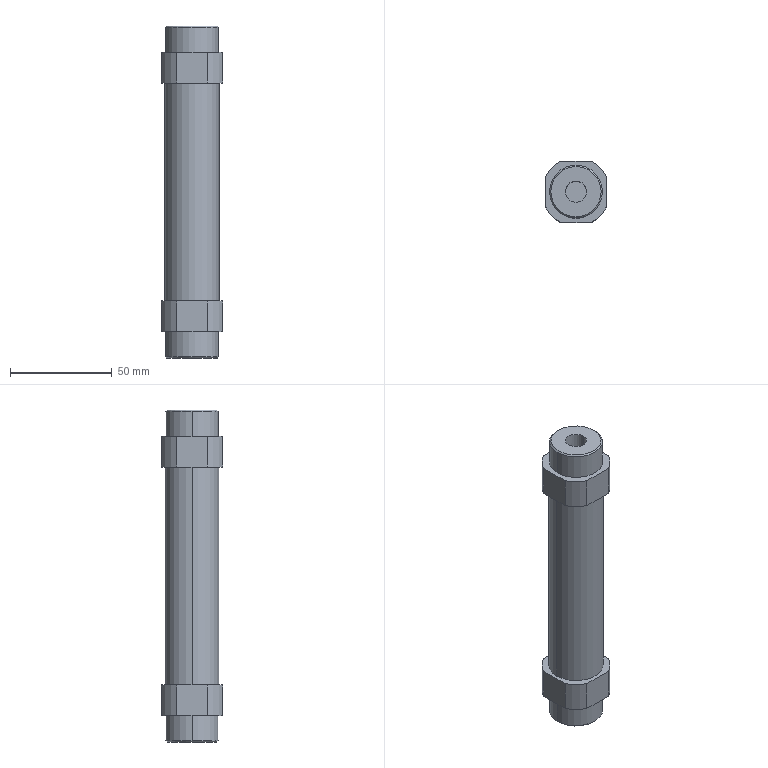Part | STEP file | 1-2 | 1 solid | 46 faces | box 30 x 30 x 163 mm | volume 89864 mm3 | cylinder 20 | plane 18 | cone 8 | commonest cylinder face diameters 33.5 x8 8.57 x4 26 x4 10.4 x2 26.6 x2
STEP:
#1=CARTESIAN_POINT('',(-13.3,0.,-28.));
#2=VERTEX_POINT('',#1);
#3=CARTESIAN_POINT('',(13.3,0.,-28.));
#4=VERTEX_POINT('',#3);
#5=CARTESIAN_POINT('',(0.,0.,-28.));
#6=DIRECTION('',(0.,0.,-1.));
#7=DIRECTION('',(-1.,0.,0.));
#8=AXIS2_PLACEMENT_3D('',#5,#6,#7);
#9=CIRCLE('',#8,13.3);
#10=EDGE_CURVE('',#2,#4,#9,.T.);
#11=ORIENTED_EDGE('',*,*,#10,.T.);
#12=CARTESIAN_POINT('',(13.3,0.,-135.));
#13=VERTEX_POINT('',#12);
#14=CARTESIAN_POINT('',(13.3,0.,-81.5));
#15=DIRECTION('',(0.,0.,-1.));
#16=VECTOR('',#15,1000.);
#17=LINE('',#14,#16);
#18=EDGE_CURVE('',#4,#13,#17,.T.);
#19=ORIENTED_EDGE('',*,*,#18,.T.);
#20=CARTESIAN_POINT('',(-13.3,0.,-135.));
#21=VERTEX_POINT('',#20);
#22=CARTESIAN_POINT('',(0.,0.,-135.));
#23=DIRECTION('',(0.,0.,1.));
#24=DIRECTION('',(-1.,0.,0.));
#25=AXIS2_PLACEMENT_3D('',#22,#23,#24);
#26=CIRCLE('',#25,13.3);
#27=EDGE_CURVE('',#13,#21,#26,.T.);
#28=ORIENTED_EDGE('',*,*,#27,.T.);
#29=CARTESIAN_POINT('',(-13.3,0.,-81.5));
#30=DIRECTION('',(0.,0.,-1.));
#31=VECTOR('',#30,1000.);
#32=LINE('',#29,#31);
#33=EDGE_CURVE('',#2,#21,#32,.T.);
#34=ORIENTED_EDGE('',*,*,#33,.F.);
#35=EDGE_LOOP('',(#11,#19,#28,#34));
#36=FACE_OUTER_BOUND('',#35,.T.);
#37=CARTESIAN_POINT('',(0.,0.,-81.5));
#38=DIRECTION('',(0.,0.,-1.));
#39=DIRECTION('',(-1.,0.,0.));
#40=AXIS2_PLACEMENT_3D('',#37,#38,#39);
#41=CYLINDRICAL_SURFACE('',#40,13.3);
#42=ADVANCED_FACE('',(#36),#41,.T.);
#43=CARTESIAN_POINT('',(0.,14.5,-25.285));
#44=VERTEX_POINT('',#43);
#45=CARTESIAN_POINT('',(0.,14.5,-16.715));
#46=VERTEX_POINT('',#45);
#47=CARTESIAN_POINT('',(0.,14.5,-21.));
#48=DIRECTION('',(0.,1.,0.));
#49=DIRECTION('',(1.,0.,0.));
#50=AXIS2_PLACEMENT_3D('',#47,#48,#49);
#51=CIRCLE('',#50,4.285);
#52=EDGE_CURVE('',#44,#46,#51,.T.);
#53=ORIENTED_EDGE('',*,*,#52,.F.);
#54=CARTESIAN_POINT('',(0.,15.,-25.785));
#55=VERTEX_POINT('',#54);
#56=CARTESIAN_POINT('',(0.,15.,-25.785));
#57=DIRECTION('',(0.,0.7071,-0.7071));
#58=VECTOR('',#57,1000.);
#59=LINE('',#56,#58);
#60=EDGE_CURVE('',#44,#55,#59,.T.);
#61=ORIENTED_EDGE('',*,*,#60,.T.);
#62=CARTESIAN_POINT('',(0.,15.,-16.215));
#63=VERTEX_POINT('',#62);
#64=CARTESIAN_POINT('',(0.,15.,-21.));
#65=DIRECTION('',(0.,-1.,0.));
#66=DIRECTION('',(0.,0.,1.));
#67=AXIS2_PLACEMENT_3D('',#64,#65,#66);
#68=CIRCLE('',#67,4.785);
#69=EDGE_CURVE('',#63,#55,#68,.T.);
#70=ORIENTED_EDGE('',*,*,#69,.F.);
#71=CARTESIAN_POINT('',(0.,15.,-16.215));
#72=DIRECTION('',(0.,0.7071,0.7071));
#73=VECTOR('',#72,1000.);
#74=LINE('',#71,#73);
#75=EDGE_CURVE('',#46,#63,#74,.T.);
#76=ORIENTED_EDGE('',*,*,#75,.F.);
#77=EDGE_LOOP('',(#53,#61,#70,#76));
#78=FACE_OUTER_BOUND('',#77,.T.);
#79=CARTESIAN_POINT('',(0.,15.,-21.));
#80=DIRECTION('',(0.,1.,0.));
#81=DIRECTION('',(0.,0.,1.));
#82=AXIS2_PLACEMENT_3D('',#79,#80,#81);
#83=CONICAL_SURFACE('',#82,4.785,0.7854);
#84=ADVANCED_FACE('',(#78),#83,.F.);
#85=CARTESIAN_POINT('',(0.,14.5,-146.285));
#86=VERTEX_POINT('',#85);
#87=CARTESIAN_POINT('',(0.,14.5,-137.715));
#88=VERTEX_POINT('',#87);
#89=CARTESIAN_POINT('',(0.,14.5,-142.));
#90=DIRECTION('',(0.,1.,0.));
#91=DIRECTION('',(1.,0.,0.));
#92=AXIS2_PLACEMENT_3D('',#89,#90,#91);
#93=CIRCLE('',#92,4.285);
#94=EDGE_CURVE('',#86,#88,#93,.T.);
#95=ORIENTED_EDGE('',*,*,#94,.F.);
#96=CARTESIAN_POINT('',(0.,15.,-146.785));
#97=VERTEX_POINT('',#96);
#98=CARTESIAN_POINT('',(0.,15.,-146.785));
#99=DIRECTION('',(0.,0.7071,-0.7071));
#100=VECTOR('',#99,1000.);
#101=LINE('',#98,#100);
#102=EDGE_CURVE('',#86,#97,#101,.T.);
#103=ORIENTED_EDGE('',*,*,#102,.T.);
#104=CARTESIAN_POINT('',(0.,15.,-137.215));
#105=VERTEX_POINT('',#104);
#106=CARTESIAN_POINT('',(0.,15.,-142.));
#107=DIRECTION('',(0.,-1.,0.));
#108=DIRECTION('',(0.,0.,1.));
#109=AXIS2_PLACEMENT_3D('',#106,#107,#108);
#110=CIRCLE('',#109,4.785);
#111=EDGE_CURVE('',#105,#97,#110,.T.);
#112=ORIENTED_EDGE('',*,*,#111,.F.);
#113=CARTESIAN_POINT('',(0.,15.,-137.215));
#114=DIRECTION('',(0.,0.7071,0.7071));
#115=VECTOR('',#114,1000.);
#116=LINE('',#113,#115);
#117=EDGE_CURVE('',#88,#105,#116,.T.);
#118=ORIENTED_EDGE('',*,*,#117,.F.);
#119=EDGE_LOOP('',(#95,#103,#112,#118));
#120=FACE_OUTER_BOUND('',#119,.T.);
#121=CARTESIAN_POINT('',(0.,15.,-142.));
#122=DIRECTION('',(0.,1.,0.));
#123=DIRECTION('',(0.,0.,1.));
#124=AXIS2_PLACEMENT_3D('',#121,#122,#123);
#125=CONICAL_SURFACE('',#124,4.785,0.7854);
#126=ADVANCED_FACE('',(#120),#125,.F.);
#127=CARTESIAN_POINT('',(-13.,0.,-0.665));
#128=VERTEX_POINT('',#127);
#129=CARTESIAN_POINT('',(13.,0.,-0.665));
#130=VERTEX_POINT('',#129);
#131=CARTESIAN_POINT('',(0.,0.,-0.665));
#132=DIRECTION('',(0.,0.,-1.));
#133=DIRECTION('',(-1.,0.,0.));
#134=AXIS2_PLACEMENT_3D('',#131,#132,#133);
#135=CIRCLE('',#134,13.);
#136=EDGE_CURVE('',#128,#130,#135,.T.);
#137=ORIENTED_EDGE('',*,*,#136,.T.);
#138=CARTESIAN_POINT('',(13.,0.,-13.));
#139=VERTEX_POINT('',#138);
#140=CARTESIAN_POINT('',(13.,0.,-7.332));
#141=DIRECTION('',(0.,0.,-1.));
#142=VECTOR('',#141,1000.);
#143=LINE('',#140,#142);
#144=EDGE_CURVE('',#130,#139,#143,.T.);
#145=ORIENTED_EDGE('',*,*,#144,.T.);
#146=CARTESIAN_POINT('',(-13.,0.,-13.));
#147=VERTEX_POINT('',#146);
#148=CARTESIAN_POINT('',(0.,0.,-13.));
#149=DIRECTION('',(0.,0.,-1.));
#150=DIRECTION('',(-1.,0.,0.));
#151=AXIS2_PLACEMENT_3D('',#148,#149,#150);
#152=CIRCLE('',#151,13.);
#153=EDGE_CURVE('',#147,#139,#152,.T.);
#154=ORIENTED_EDGE('',*,*,#153,.F.);
#155=CARTESIAN_POINT('',(-13.,0.,-7.332));
#156=DIRECTION('',(0.,0.,-1.));
#157=VECTOR('',#156,1000.);
#158=LINE('',#155,#157);
#159=EDGE_CURVE('',#128,#147,#158,.T.);
#160=ORIENTED_EDGE('',*,*,#159,.F.);
#161=EDGE_LOOP('',(#137,#145,#154,#160));
#162=FACE_OUTER_BOUND('',#161,.T.);
#163=CARTESIAN_POINT('',(0.,0.,-7.332));
#164=DIRECTION('',(0.,0.,-1.));
#165=DIRECTION('',(-1.,0.,0.));
#166=AXIS2_PLACEMENT_3D('',#163,#164,#165);
#167=CYLINDRICAL_SURFACE('',#166,13.);
#168=ADVANCED_FACE('',(#162),#167,.T.);
#169=ORIENTED_EDGE('',*,*,#52,.T.);
#170=CARTESIAN_POINT('',(0.,5.2,-16.715));
#171=VERTEX_POINT('',#170);
#172=CARTESIAN_POINT('',(0.,9.75,-16.715));
#173=DIRECTION('',(0.,-1.,0.));
#174=VECTOR('',#173,1000.);
#175=LINE('',#172,#174);
#176=EDGE_CURVE('',#46,#171,#175,.T.);
#177=ORIENTED_EDGE('',*,*,#176,.T.);
#178=CARTESIAN_POINT('',(-1.428,5.,-16.96));
#179=VERTEX_POINT('',#178);
#180=CARTESIAN_POINT('',(-1.428,5.,-16.96));
#181=CARTESIAN_POINT('',(-1.203,5.064,-16.88));
#182=CARTESIAN_POINT('',(-0.9709,5.114,-16.819));
#183=CARTESIAN_POINT('',(-0.4935,5.182,-16.737));
#184=CARTESIAN_POINT('',(-0.2449,5.2,-16.715));
#185=CARTESIAN_POINT('',(0.,5.2,-16.715));
#186=B_SPLINE_CURVE_WITH_KNOTS('',3,(#180,#181,#182,#183,#184,#185),.UNSPECIFIED.,.F.,.F.,(4,2,4),(0.,0.0007333,0.001467),.UNSPECIFIED.);
#187=EDGE_CURVE('',#179,#171,#186,.T.);
#188=ORIENTED_EDGE('',*,*,#187,.F.);
#189=CARTESIAN_POINT('',(-1.428,5.,-25.04));
#190=VERTEX_POINT('',#189);
#191=CARTESIAN_POINT('',(0.,5.,-21.));
#192=DIRECTION('',(0.,1.,0.));
#193=DIRECTION('',(0.,0.,-1.));
#194=AXIS2_PLACEMENT_3D('',#191,#192,#193);
#195=CIRCLE('',#194,4.285);
#196=EDGE_CURVE('',#190,#179,#195,.T.);
#197=ORIENTED_EDGE('',*,*,#196,.F.);
#198=CARTESIAN_POINT('',(0.,5.2,-25.285));
#199=VERTEX_POINT('',#198);
#200=CARTESIAN_POINT('',(0.,5.2,-25.285));
#201=CARTESIAN_POINT('',(-0.2446,5.2,-25.285));
#202=CARTESIAN_POINT('',(-0.4871,5.183,-25.264));
#203=CARTESIAN_POINT('',(-0.9681,5.115,-25.181));
#204=CARTESIAN_POINT('',(-1.203,5.064,-25.12));
#205=CARTESIAN_POINT('',(-1.428,5.,-25.04));
#206=B_SPLINE_CURVE_WITH_KNOTS('',3,(#200,#201,#202,#203,#204,#205),.UNSPECIFIED.,.F.,.F.,(4,2,4),(0.001467,0.002199,0.002931),.UNSPECIFIED.);
#207=EDGE_CURVE('',#199,#190,#206,.T.);
#208=ORIENTED_EDGE('',*,*,#207,.F.);
#209=CARTESIAN_POINT('',(0.,9.75,-25.285));
#210=DIRECTION('',(0.,-1.,0.));
#211=VECTOR('',#210,1000.);
#212=LINE('',#209,#211);
#213=EDGE_CURVE('',#44,#199,#212,.T.);
#214=ORIENTED_EDGE('',*,*,#213,.F.);
#215=EDGE_LOOP('',(#169,#177,#188,#197,#208,#214));
#216=FACE_OUTER_BOUND('',#215,.T.);
#217=CARTESIAN_POINT('',(0.,9.75,-21.));
#218=DIRECTION('',(0.,-1.,0.));
#219=DIRECTION('',(0.,0.,-1.));
#220=AXIS2_PLACEMENT_3D('',#217,#218,#219);
#221=CYLINDRICAL_SURFACE('',#220,4.285);
#222=ADVANCED_FACE('',(#216),#221,.F.);
#223=CARTESIAN_POINT('',(-13.,0.,-150.));
#224=VERTEX_POINT('',#223);
#225=CARTESIAN_POINT('',(13.,0.,-150.));
#226=VERTEX_POINT('',#225);
#227=CARTESIAN_POINT('',(0.,0.,-150.));
#228=DIRECTION('',(0.,0.,-1.));
#229=DIRECTION('',(-1.,0.,0.));
#230=AXIS2_PLACEMENT_3D('',#227,#228,#229);
#231=CIRCLE('',#230,13.);
#232=EDGE_CURVE('',#224,#226,#231,.T.);
#233=ORIENTED_EDGE('',*,*,#232,.T.);
#234=CARTESIAN_POINT('',(13.,0.,-162.335));
#235=VERTEX_POINT('',#234);
#236=CARTESIAN_POINT('',(13.,0.,-155.667));
#237=DIRECTION('',(0.,0.,-1.));
#238=VECTOR('',#237,1000.);
#239=LINE('',#236,#238);
#240=EDGE_CURVE('',#226,#235,#239,.T.);
#241=ORIENTED_EDGE('',*,*,#240,.T.);
#242=CARTESIAN_POINT('',(-13.,0.,-162.335));
#243=VERTEX_POINT('',#242);
#244=CARTESIAN_POINT('',(0.,0.,-162.335));
#245=DIRECTION('',(0.,0.,1.));
#246=DIRECTION('',(-1.,0.,0.));
#247=AXIS2_PLACEMENT_3D('',#244,#245,#246);
#248=CIRCLE('',#247,13.);
#249=EDGE_CURVE('',#235,#243,#248,.T.);
#250=ORIENTED_EDGE('',*,*,#249,.T.);
#251=CARTESIAN_POINT('',(-13.,0.,-155.667));
#252=DIRECTION('',(0.,0.,-1.));
#253=VECTOR('',#252,1000.);
#254=LINE('',#251,#253);
#255=EDGE_CURVE('',#224,#243,#254,.T.);
#256=ORIENTED_EDGE('',*,*,#255,.F.);
#257=EDGE_LOOP('',(#233,#241,#250,#256));
#258=FACE_OUTER_BOUND('',#257,.T.);
#259=CARTESIAN_POINT('',(0.,0.,-155.667));
#260=DIRECTION('',(0.,0.,-1.));
#261=DIRECTION('',(-1.,0.,0.));
#262=AXIS2_PLACEMENT_3D('',#259,#260,#261);
#263=CYLINDRICAL_SURFACE('',#262,13.);
#264=ADVANCED_FACE('',(#258),#263,.T.);
#265=ORIENTED_EDGE('',*,*,#94,.T.);
#266=CARTESIAN_POINT('',(0.,5.,-137.715));
#267=VERTEX_POINT('',#266);
#268=CARTESIAN_POINT('',(0.,9.75,-137.715));
#269=DIRECTION('',(0.,-1.,0.));
#270=VECTOR('',#269,1000.);
#271=LINE('',#268,#270);
#272=EDGE_CURVE('',#88,#267,#271,.T.);
#273=ORIENTED_EDGE('',*,*,#272,.T.);
#274=CARTESIAN_POINT('',(0.,5.,-146.285));
#275=VERTEX_POINT('',#274);
#276=CARTESIAN_POINT('',(0.,5.,-142.));
#277=DIRECTION('',(0.,1.,0.));
#278=DIRECTION('',(0.,0.,-1.));
#279=AXIS2_PLACEMENT_3D('',#276,#277,#278);
#280=CIRCLE('',#279,4.285);
#281=EDGE_CURVE('',#275,#267,#280,.T.);
#282=ORIENTED_EDGE('',*,*,#281,.F.);
#283=CARTESIAN_POINT('',(0.,9.75,-146.285));
#284=DIRECTION('',(0.,-1.,0.));
#285=VECTOR('',#284,1000.);
#286=LINE('',#283,#285);
#287=EDGE_CURVE('',#86,#275,#286,.T.);
#288=ORIENTED_EDGE('',*,*,#287,.F.);
#289=EDGE_LOOP('',(#265,#273,#282,#288));
#290=FACE_OUTER_BOUND('',#289,.T.);
#291=CARTESIAN_POINT('',(0.,9.75,-142.));
#292=DIRECTION('',(0.,-1.,0.));
#293=DIRECTION('',(0.,0.,-1.));
#294=AXIS2_PLACEMENT_3D('',#291,#292,#293);
#295=CYLINDRICAL_SURFACE('',#294,4.285);
#296=ADVANCED_FACE('',(#290),#295,.F.);
#297=CARTESIAN_POINT('',(-12.335,0.,0.));
#298=VERTEX_POINT('',#297);
#299=CARTESIAN_POINT('',(12.335,0.,0.));
#300=VERTEX_POINT('',#299);
#301=CARTESIAN_POINT('',(0.,0.,0.));
#302=DIRECTION('',(0.,0.,-1.));
#303=DIRECTION('',(-1.,0.,0.));
#304=AXIS2_PLACEMENT_3D('',#301,#302,#303);
#305=CIRCLE('',#304,12.335);
#306=EDGE_CURVE('',#298,#300,#305,.T.);
#307=ORIENTED_EDGE('',*,*,#306,.T.);
#308=CARTESIAN_POINT('',(13.,0.,-0.665));
#309=DIRECTION('',(0.7071,0.,-0.7071));
#310=VECTOR('',#309,1000.);
#311=LINE('',#308,#310);
#312=EDGE_CURVE('',#300,#130,#311,.T.);
#313=ORIENTED_EDGE('',*,*,#312,.T.);
#314=ORIENTED_EDGE('',*,*,#136,.F.);
#315=CARTESIAN_POINT('',(-13.,0.,-0.665));
#316=DIRECTION('',(-0.7071,0.,-0.7071));
#317=VECTOR('',#316,1000.);
#318=LINE('',#315,#317);
#319=EDGE_CURVE('',#298,#128,#318,.T.);
#320=ORIENTED_EDGE('',*,*,#319,.F.);
#321=EDGE_LOOP('',(#307,#313,#314,#320));
#322=FACE_OUTER_BOUND('',#321,.T.);
#323=CARTESIAN_POINT('',(0.,0.,-0.665));
#324=DIRECTION('',(0.,0.,-1.));
#325=DIRECTION('',(-1.,0.,0.));
#326=AXIS2_PLACEMENT_3D('',#323,#324,#325);
#327=CONICAL_SURFACE('',#326,13.,0.7854);
#328=ADVANCED_FACE('',(#322),#327,.T.);
#329=CARTESIAN_POINT('',(-5.2,0.,-77.));
#330=VERTEX_POINT('',#329);
#331=CARTESIAN_POINT('',(5.2,0.,-77.));
#332=VERTEX_POINT('',#331);
#333=CARTESIAN_POINT('',(0.,0.,-77.));
#334=DIRECTION('',(0.,0.,1.));
#335=DIRECTION('',(1.,0.,0.));
#336=AXIS2_PLACEMENT_3D('',#333,#334,#335);
#337=CIRCLE('',#336,5.2);
#338=EDGE_CURVE('',#330,#332,#337,.T.);
#339=ORIENTED_EDGE('',*,*,#338,.F.);
#340=CARTESIAN_POINT('',(-5.2,0.,0.));
#341=VERTEX_POINT('',#340);
#342=CARTESIAN_POINT('',(-5.2,0.,0.));
#343=DIRECTION('',(0.,0.,1.));
#344=VECTOR('',#343,1000.);
#345=LINE('',#342,#344);
#346=EDGE_CURVE('',#330,#341,#345,.T.);
#347=ORIENTED_EDGE('',*,*,#346,.T.);
#348=CARTESIAN_POINT('',(5.2,0.,0.));
#349=VERTEX_POINT('',#348);
#350=CARTESIAN_POINT('',(0.,0.,0.));
#351=DIRECTION('',(0.,0.,-1.));
#352=DIRECTION('',(1.,0.,0.));
#353=AXIS2_PLACEMENT_3D('',#350,#351,#352);
#354=CIRCLE('',#353,5.2);
#355=EDGE_CURVE('',#349,#341,#354,.T.);
#356=ORIENTED_EDGE('',*,*,#355,.F.);
#357=CARTESIAN_POINT('',(5.2,0.,0.));
#358=DIRECTION('',(0.,0.,1.));
#359=VECTOR('',#358,1000.);
#360=LINE('',#357,#359);
#361=EDGE_CURVE('',#332,#349,#360,.T.);
#362=ORIENTED_EDGE('',*,*,#361,.F.);
#363=EDGE_LOOP('',(#339,#347,#356,#362));
#364=FACE_OUTER_BOUND('',#363,.T.);
#365=CARTESIAN_POINT('',(0.,0.,0.));
#366=DIRECTION('',(0.,0.,1.));
#367=DIRECTION('',(1.,0.,0.));
#368=AXIS2_PLACEMENT_3D('',#365,#366,#367);
#369=CYLINDRICAL_SURFACE('',#368,5.2);
#370=ADVANCED_FACE('',(#364),#369,.F.);
#371=CARTESIAN_POINT('',(12.335,0.,-163.));
#372=VERTEX_POINT('',#371);
#373=CARTESIAN_POINT('',(-12.335,0.,-163.));
#374=VERTEX_POINT('',#373);
#375=CARTESIAN_POINT('',(0.,0.,-163.));
#376=DIRECTION('',(0.,0.,1.));
#377=DIRECTION('',(1.,0.,0.));
#378=AXIS2_PLACEMENT_3D('',#375,#376,#377);
#379=CIRCLE('',#378,12.335);
#380=EDGE_CURVE('',#372,#374,#379,.T.);
#381=ORIENTED_EDGE('',*,*,#380,.T.);
#382=CARTESIAN_POINT('',(-13.,0.,-162.335));
#383=DIRECTION('',(-0.7071,0.,0.7071));
#384=VECTOR('',#383,1000.);
#385=LINE('',#382,#384);
#386=EDGE_CURVE('',#374,#243,#385,.T.);
#387=ORIENTED_EDGE('',*,*,#386,.T.);
#388=ORIENTED_EDGE('',*,*,#249,.F.);
#389=CARTESIAN_POINT('',(13.,0.,-162.335));
#390=DIRECTION('',(0.7071,0.,0.7071));
#391=VECTOR('',#390,1000.);
#392=LINE('',#389,#391);
#393=EDGE_CURVE('',#372,#235,#392,.T.);
#394=ORIENTED_EDGE('',*,*,#393,.F.);
#395=EDGE_LOOP('',(#381,#387,#388,#394));
#396=FACE_OUTER_BOUND('',#395,.T.);
#397=CARTESIAN_POINT('',(0.,0.,-162.335));
#398=DIRECTION('',(0.,0.,1.));
#399=DIRECTION('',(1.,0.,0.));
#400=AXIS2_PLACEMENT_3D('',#397,#398,#399);
#401=CONICAL_SURFACE('',#400,13.,0.7854);
#402=ADVANCED_FACE('',(#396),#401,.T.);
#403=ORIENTED_EDGE('',*,*,#18,.F.);
#404=CARTESIAN_POINT('',(0.,0.,-28.));
#405=DIRECTION('',(0.,0.,-1.));
#406=DIRECTION('',(-1.,0.,0.));
#407=AXIS2_PLACEMENT_3D('',#404,#405,#406);
#408=CIRCLE('',#407,13.3);
#409=EDGE_CURVE('',#4,#2,#408,.T.);
#410=ORIENTED_EDGE('',*,*,#409,.T.);
#411=ORIENTED_EDGE('',*,*,#33,.T.);
#412=CARTESIAN_POINT('',(0.,0.,-135.));
#413=DIRECTION('',(0.,0.,1.));
#414=DIRECTION('',(-1.,0.,0.));
#415=AXIS2_PLACEMENT_3D('',#412,#413,#414);
#416=CIRCLE('',#415,13.3);
#417=EDGE_CURVE('',#21,#13,#416,.T.);
#418=ORIENTED_EDGE('',*,*,#417,.T.);
#419=EDGE_LOOP('',(#403,#410,#411,#418));
#420=FACE_OUTER_BOUND('',#419,.T.);
#421=CARTESIAN_POINT('',(0.,0.,-81.5));
#422=DIRECTION('',(0.,0.,-1.));
#423=DIRECTION('',(-1.,0.,0.));
#424=AXIS2_PLACEMENT_3D('',#421,#422,#423);
#425=CYLINDRICAL_SURFACE('',#424,13.3);
#426=ADVANCED_FACE('',(#420),#425,.T.);
#427=ORIENTED_EDGE('',*,*,#10,.F.);
#428=ORIENTED_EDGE('',*,*,#409,.F.);
#429=EDGE_LOOP('',(#427,#428));
#430=FACE_BOUND('',#429,.T.);
#431=CARTESIAN_POINT('',(-15.,-7.454,-28.));
#432=VERTEX_POINT('',#431);
#433=CARTESIAN_POINT('',(-7.454,-15.,-28.));
#434=VERTEX_POINT('',#433);
#435=CARTESIAN_POINT('',(0.,0.,-28.));
#436=DIRECTION('',(0.,0.,1.));
#437=DIRECTION('',(1.,0.,0.));
#438=AXIS2_PLACEMENT_3D('',#435,#436,#437);
#439=CIRCLE('',#438,16.75);
#440=EDGE_CURVE('',#432,#434,#439,.T.);
#441=ORIENTED_EDGE('',*,*,#440,.F.);
#442=CARTESIAN_POINT('',(-15.,7.454,-28.));
#443=VERTEX_POINT('',#442);
#444=CARTESIAN_POINT('',(-15.,0.,-28.));
#445=DIRECTION('',(0.,-1.,0.));
#446=VECTOR('',#445,1000.);
#447=LINE('',#444,#446);
#448=EDGE_CURVE('',#443,#432,#447,.T.);
#449=ORIENTED_EDGE('',*,*,#448,.F.);
#450=CARTESIAN_POINT('',(-7.454,15.,-28.));
#451=VERTEX_POINT('',#450);
#452=CARTESIAN_POINT('',(0.,0.,-28.));
#453=DIRECTION('',(0.,0.,1.));
#454=DIRECTION('',(1.,0.,0.));
#455=AXIS2_PLACEMENT_3D('',#452,#453,#454);
#456=CIRCLE('',#455,16.75);
#457=EDGE_CURVE('',#451,#443,#456,.T.);
#458=ORIENTED_EDGE('',*,*,#457,.F.);
#459=CARTESIAN_POINT('',(7.454,15.,-28.));
#460=VERTEX_POINT('',#459);
#461=CARTESIAN_POINT('',(0.,15.,-28.));
#462=DIRECTION('',(-1.,0.,0.));
#463=VECTOR('',#462,1000.);
#464=LINE('',#461,#463);
#465=EDGE_CURVE('',#460,#451,#464,.T.);
#466=ORIENTED_EDGE('',*,*,#465,.F.);
#467=CARTESIAN_POINT('',(15.,7.454,-28.));
#468=VERTEX_POINT('',#467);
#469=CARTESIAN_POINT('',(0.,0.,-28.));
#470=DIRECTION('',(0.,0.,1.));
#471=DIRECTION('',(1.,0.,0.));
#472=AXIS2_PLACEMENT_3D('',#469,#470,#471);
#473=CIRCLE('',#472,16.75);
#474=EDGE_CURVE('',#468,#460,#473,.T.);
#475=ORIENTED_EDGE('',*,*,#474,.F.);
#476=CARTESIAN_POINT('',(15.,-7.454,-28.));
#477=VERTEX_POINT('',#476);
#478=CARTESIAN_POINT('',(15.,0.,-28.));
#479=DIRECTION('',(0.,1.,0.));
#480=VECTOR('',#479,1000.);
#481=LINE('',#478,#480);
#482=EDGE_CURVE('',#477,#468,#481,.T.);
#483=ORIENTED_EDGE('',*,*,#482,.F.);
#484=CARTESIAN_POINT('',(7.454,-15.,-28.));
#485=VERTEX_POINT('',#484);
#486=CARTESIAN_POINT('',(0.,0.,-28.));
#487=DIRECTION('',(0.,0.,1.));
#488=DIRECTION('',(1.,0.,0.));
#489=AXIS2_PLACEMENT_3D('',#486,#487,#488);
#490=CIRCLE('',#489,16.75);
#491=EDGE_CURVE('',#485,#477,#490,.T.);
#492=ORIENTED_EDGE('',*,*,#491,.F.);
#493=CARTESIAN_POINT('',(0.,-15.,-28.));
#494=DIRECTION('',(1.,0.,0.));
#495=VECTOR('',#494,1000.);
#496=LINE('',#493,#495);
#497=EDGE_CURVE('',#434,#485,#496,.T.);
#498=ORIENTED_EDGE('',*,*,#497,.F.);
#499=EDGE_LOOP('',(#441,#449,#458,#466,#475,#483,#492,#498));
#500=FACE_OUTER_BOUND('',#499,.T.);
#501=CARTESIAN_POINT('',(0.,0.,-28.));
#502=DIRECTION('',(0.,0.,1.));
#503=DIRECTION('',(1.,0.,0.));
#504=AXIS2_PLACEMENT_3D('',#501,#502,#503);
#505=PLANE('',#504);
#506=ADVANCED_FACE('',(#430,#500),#505,.F.);
#507=ORIENTED_EDGE('',*,*,#417,.F.);
#508=ORIENTED_EDGE('',*,*,#27,.F.);
#509=EDGE_LOOP('',(#507,#508));
#510=FACE_BOUND('',#509,.T.);
#511=CARTESIAN_POINT('',(7.454,15.,-135.));
#512=VERTEX_POINT('',#511);
#513=CARTESIAN_POINT('',(-7.454,15.,-135.));
#514=VERTEX_POINT('',#513);
#515=CARTESIAN_POINT('',(0.,15.,-135.));
#516=DIRECTION('',(-1.,0.,0.));
#517=VECTOR('',#516,1000.);
#518=LINE('',#515,#517);
#519=EDGE_CURVE('',#512,#514,#518,.T.);
#520=ORIENTED_EDGE('',*,*,#519,.T.);
#521=CARTESIAN_POINT('',(-15.,7.454,-135.));
#522=VERTEX_POINT('',#521);
#523=CARTESIAN_POINT('',(0.,0.,-135.));
#524=DIRECTION('',(0.,0.,1.));
#525=DIRECTION('',(-1.,0.,0.));
#526=AXIS2_PLACEMENT_3D('',#523,#524,#525);
#527=CIRCLE('',#526,16.75);
#528=EDGE_CURVE('',#514,#522,#527,.T.);
#529=ORIENTED_EDGE('',*,*,#528,.T.);
#530=CARTESIAN_POINT('',(-15.,-7.454,-135.));
#531=VERTEX_POINT('',#530);
#532=CARTESIAN_POINT('',(-15.,0.,-135.));
#533=DIRECTION('',(0.,-1.,0.));
#534=VECTOR('',#533,1000.);
#535=LINE('',#532,#534);
#536=EDGE_CURVE('',#522,#531,#535,.T.);
#537=ORIENTED_EDGE('',*,*,#536,.T.);
#538=CARTESIAN_POINT('',(-7.454,-15.,-135.));
#539=VERTEX_POINT('',#538);
#540=CARTESIAN_POINT('',(0.,0.,-135.));
#541=DIRECTION('',(0.,0.,1.));
#542=DIRECTION('',(-1.,0.,0.));
#543=AXIS2_PLACEMENT_3D('',#540,#541,#542);
#544=CIRCLE('',#543,16.75);
#545=EDGE_CURVE('',#531,#539,#544,.T.);
#546=ORIENTED_EDGE('',*,*,#545,.T.);
#547=CARTESIAN_POINT('',(7.454,-15.,-135.));
#548=VERTEX_POINT('',#547);
#549=CARTESIAN_POINT('',(0.,-15.,-135.));
#550=DIRECTION('',(1.,0.,0.));
#551=VECTOR('',#550,1000.);
#552=LINE('',#549,#551);
#553=EDGE_CURVE('',#539,#548,#552,.T.);
#554=ORIENTED_EDGE('',*,*,#553,.T.);
#555=CARTESIAN_POINT('',(15.,-7.454,-135.));
#556=VERTEX_POINT('',#555);
#557=CARTESIAN_POINT('',(0.,0.,-135.));
#558=DIRECTION('',(0.,0.,1.));
#559=DIRECTION('',(-1.,0.,0.));
#560=AXIS2_PLACEMENT_3D('',#557,#558,#559);
#561=CIRCLE('',#560,16.75);
#562=EDGE_CURVE('',#548,#556,#561,.T.);
#563=ORIENTED_EDGE('',*,*,#562,.T.);
#564=CARTESIAN_POINT('',(15.,7.454,-135.));
#565=VERTEX_POINT('',#564);
#566=CARTESIAN_POINT('',(15.,0.,-135.));
#567=DIRECTION('',(0.,1.,0.));
#568=VECTOR('',#567,1000.);
#569=LINE('',#566,#568);
#570=EDGE_CURVE('',#556,#565,#569,.T.);
#571=ORIENTED_EDGE('',*,*,#570,.T.);
#572=CARTESIAN_POINT('',(0.,0.,-135.));
#573=DIRECTION('',(0.,0.,1.));
#574=DIRECTION('',(-1.,0.,0.));
#575=AXIS2_PLACEMENT_3D('',#572,#573,#574);
#576=CIRCLE('',#575,16.75);
#577=EDGE_CURVE('',#565,#512,#576,.T.);
#578=ORIENTED_EDGE('',*,*,#577,.T.);
#579=EDGE_LOOP('',(#520,#529,#537,#546,#554,#563,#571,#578));
#580=FACE_OUTER_BOUND('',#579,.T.);
#581=CARTESIAN_POINT('',(0.,0.,-135.));
#582=DIRECTION('',(0.,0.,1.));
#583=DIRECTION('',(1.,0.,0.));
#584=AXIS2_PLACEMENT_3D('',#581,#582,#583);
#585=PLANE('',#584);
#586=ADVANCED_FACE('',(#510,#580),#585,.T.);
#587=CARTESIAN_POINT('',(7.454,-15.,-13.));
#588=VERTEX_POINT('',#587);
#589=CARTESIAN_POINT('',(-7.454,-15.,-13.));
#590=VERTEX_POINT('',#589);
#591=CARTESIAN_POINT('',(-7.454,-15.,-13.));
#592=DIRECTION('',(-1.,0.,0.));
#593=VECTOR('',#592,1000.);
#594=LINE('',#591,#593);
#595=EDGE_CURVE('',#588,#590,#594,.T.);
#596=ORIENTED_EDGE('',*,*,#595,.T.);
#597=CARTESIAN_POINT('',(-7.454,-15.,-13.));
#598=DIRECTION('',(0.,0.,-1.));
#599=VECTOR('',#598,1000.);
#600=LINE('',#597,#599);
#601=EDGE_CURVE('',#590,#434,#600,.T.);
#602=ORIENTED_EDGE('',*,*,#601,.T.);
#603=ORIENTED_EDGE('',*,*,#497,.T.);
#604=CARTESIAN_POINT('',(7.454,-15.,-13.));
#605=DIRECTION('',(0.,0.,1.));
#606=VECTOR('',#605,1000.);
#607=LINE('',#604,#606);
#608=EDGE_CURVE('',#485,#588,#607,.T.);
#609=ORIENTED_EDGE('',*,*,#608,.T.);
#610=EDGE_LOOP('',(#596,#602,#603,#609));
#611=FACE_OUTER_BOUND('',#610,.T.);
#612=CARTESIAN_POINT('',(-7.454,-15.,-13.));
#613=DIRECTION('',(0.,-1.,0.));
#614=DIRECTION('',(0.,0.,-1.));
#615=AXIS2_PLACEMENT_3D('',#612,#613,#614);
#616=PLANE('',#615);
#617=ADVANCED_FACE('',(#611),#616,.T.);
#618=CARTESIAN_POINT('',(-15.,-7.454,-13.));
#619=VERTEX_POINT('',#618);
#620=CARTESIAN_POINT('',(0.,0.,-13.));
#621=DIRECTION('',(0.,0.,-1.));
#622=DIRECTION('',(1.,0.,0.));
#623=AXIS2_PLACEMENT_3D('',#620,#621,#622);
#624=CIRCLE('',#623,16.75);
#625=EDGE_CURVE('',#590,#619,#624,.T.);
#626=ORIENTED_EDGE('',*,*,#625,.T.);
#627=CARTESIAN_POINT('',(-15.,-7.454,-13.));
#628=DIRECTION('',(0.,0.,-1.));
#629=VECTOR('',#628,1000.);
#630=LINE('',#627,#629);
#631=EDGE_CURVE('',#619,#432,#630,.T.);
#632=ORIENTED_EDGE('',*,*,#631,.T.);
#633=ORIENTED_EDGE('',*,*,#440,.T.);
#634=ORIENTED_EDGE('',*,*,#601,.F.);
#635=EDGE_LOOP('',(#626,#632,#633,#634));
#636=FACE_OUTER_BOUND('',#635,.T.);
#637=CARTESIAN_POINT('',(0.,0.,-13.));
#638=DIRECTION('',(0.,0.,1.));
#639=DIRECTION('',(1.,0.,0.));
#640=AXIS2_PLACEMENT_3D('',#637,#638,#639);
#641=CYLINDRICAL_SURFACE('',#640,16.75);
#642=ADVANCED_FACE('',(#636),#641,.T.);
#643=CARTESIAN_POINT('',(-15.,7.454,-13.));
#644=VERTEX_POINT('',#643);
#645=CARTESIAN_POINT('',(-15.,7.454,-13.));
#646=DIRECTION('',(0.,1.,0.));
#647=VECTOR('',#646,1000.);
#648=LINE('',#645,#647);
#649=EDGE_CURVE('',#619,#644,#648,.T.);
#650=ORIENTED_EDGE('',*,*,#649,.T.);
#651=CARTESIAN_POINT('',(-15.,7.454,-13.));
#652=DIRECTION('',(0.,0.,-1.));
#653=VECTOR('',#652,1000.);
#654=LINE('',#651,#653);
#655=EDGE_CURVE('',#644,#443,#654,.T.);
#656=ORIENTED_EDGE('',*,*,#655,.T.);
#657=ORIENTED_EDGE('',*,*,#448,.T.);
#658=ORIENTED_EDGE('',*,*,#631,.F.);
#659=EDGE_LOOP('',(#650,#656,#657,#658));
#660=FACE_OUTER_BOUND('',#659,.T.);
#661=CARTESIAN_POINT('',(-15.,7.454,-13.));
#662=DIRECTION('',(-1.,0.,0.));
#663=DIRECTION('',(0.,0.,1.));
#664=AXIS2_PLACEMENT_3D('',#661,#662,#663);
#665=PLANE('',#664);
#666=ADVANCED_FACE('',(#660),#665,.T.);
#667=CARTESIAN_POINT('',(-7.454,15.,-13.));
#668=VERTEX_POINT('',#667);
#669=CARTESIAN_POINT('',(0.,0.,-13.));
#670=DIRECTION('',(0.,0.,-1.));
#671=DIRECTION('',(1.,0.,0.));
#672=AXIS2_PLACEMENT_3D('',#669,#670,#671);
#673=CIRCLE('',#672,16.75);
#674=EDGE_CURVE('',#644,#668,#673,.T.);
#675=ORIENTED_EDGE('',*,*,#674,.T.);
#676=CARTESIAN_POINT('',(-7.454,15.,-13.));
#677=DIRECTION('',(0.,0.,-1.));
#678=VECTOR('',#677,1000.);
#679=LINE('',#676,#678);
#680=EDGE_CURVE('',#668,#451,#679,.T.);
#681=ORIENTED_EDGE('',*,*,#680,.T.);
#682=ORIENTED_EDGE('',*,*,#457,.T.);
#683=ORIENTED_EDGE('',*,*,#655,.F.);
#684=EDGE_LOOP('',(#675,#681,#682,#683));
#685=FACE_OUTER_BOUND('',#684,.T.);
#686=CARTESIAN_POINT('',(0.,0.,-13.));
#687=DIRECTION('',(0.,0.,1.));
#688=DIRECTION('',(1.,0.,0.));
#689=AXIS2_PLACEMENT_3D('',#686,#687,#688);
#690=CYLINDRICAL_SURFACE('',#689,16.75);
#691=ADVANCED_FACE('',(#685),#690,.T.);
#692=CARTESIAN_POINT('',(7.454,15.,-13.));
#693=VERTEX_POINT('',#692);
#694=CARTESIAN_POINT('',(7.454,15.,-13.));
#695=DIRECTION('',(1.,0.,0.));
#696=VECTOR('',#695,1000.);
#697=LINE('',#694,#696);
#698=EDGE_CURVE('',#668,#693,#697,.T.);
#699=ORIENTED_EDGE('',*,*,#698,.T.);
#700=CARTESIAN_POINT('',(7.454,15.,-13.));
#701=DIRECTION('',(0.,0.,-1.));
#702=VECTOR('',#701,1000.);
#703=LINE('',#700,#702);
#704=EDGE_CURVE('',#693,#460,#703,.T.);
#705=ORIENTED_EDGE('',*,*,#704,.T.);
#706=ORIENTED_EDGE('',*,*,#465,.T.);
#707=ORIENTED_EDGE('',*,*,#680,.F.);
#708=EDGE_LOOP('',(#699,#705,#706,#707));
#709=FACE_OUTER_BOUND('',#708,.T.);
#710=ORIENTED_EDGE('',*,*,#69,.T.);
#711=CARTESIAN_POINT('',(0.,15.,-21.));
#712=DIRECTION('',(0.,-1.,0.));
#713=DIRECTION('',(0.,0.,1.));
#714=AXIS2_PLACEMENT_3D('',#711,#712,#713);
#715=CIRCLE('',#714,4.785);
#716=EDGE_CURVE('',#55,#63,#715,.T.);
#717=ORIENTED_EDGE('',*,*,#716,.T.);
#718=EDGE_LOOP('',(#710,#717));
#719=FACE_BOUND('',#718,.T.);
#720=CARTESIAN_POINT('',(7.454,15.,-13.));
#721=DIRECTION('',(0.,1.,0.));
#722=DIRECTION('',(0.,0.,1.));
#723=AXIS2_PLACEMENT_3D('',#720,#721,#722);
#724=PLANE('',#723);
#725=ADVANCED_FACE('',(#709,#719),#724,.T.);
#726=CARTESIAN_POINT('',(15.,7.454,-13.));
#727=VERTEX_POINT('',#726);
#728=CARTESIAN_POINT('',(0.,0.,-13.));
#729=DIRECTION('',(0.,0.,-1.));
#730=DIRECTION('',(1.,0.,0.));
#731=AXIS2_PLACEMENT_3D('',#728,#729,#730);
#732=CIRCLE('',#731,16.75);
#733=EDGE_CURVE('',#693,#727,#732,.T.);
#734=ORIENTED_EDGE('',*,*,#733,.T.);
#735=CARTESIAN_POINT('',(15.,7.454,-13.));
#736=DIRECTION('',(0.,0.,-1.));
#737=VECTOR('',#736,1000.);
#738=LINE('',#735,#737);
#739=EDGE_CURVE('',#727,#468,#738,.T.);
#740=ORIENTED_EDGE('',*,*,#739,.T.);
#741=ORIENTED_EDGE('',*,*,#474,.T.);
#742=ORIENTED_EDGE('',*,*,#704,.F.);
#743=EDGE_LOOP('',(#734,#740,#741,#742));
#744=FACE_OUTER_BOUND('',#743,.T.);
#745=CARTESIAN_POINT('',(0.,0.,-13.));
#746=DIRECTION('',(0.,0.,1.));
#747=DIRECTION('',(1.,0.,0.));
#748=AXIS2_PLACEMENT_3D('',#745,#746,#747);
#749=CYLINDRICAL_SURFACE('',#748,16.75);
#750=ADVANCED_FACE('',(#744),#749,.T.);
#751=CARTESIAN_POINT('',(15.,-7.454,-13.));
#752=VERTEX_POINT('',#751);
#753=CARTESIAN_POINT('',(15.,-7.454,-13.));
#754=DIRECTION('',(0.,-1.,0.));
#755=VECTOR('',#754,1000.);
#756=LINE('',#753,#755);
#757=EDGE_CURVE('',#727,#752,#756,.T.);
#758=ORIENTED_EDGE('',*,*,#757,.T.);
#759=CARTESIAN_POINT('',(15.,-7.454,-13.));
#760=DIRECTION('',(0.,0.,-1.));
#761=VECTOR('',#760,1000.);
#762=LINE('',#759,#761);
#763=EDGE_CURVE('',#752,#477,#762,.T.);
#764=ORIENTED_EDGE('',*,*,#763,.T.);
#765=ORIENTED_EDGE('',*,*,#482,.T.);
#766=ORIENTED_EDGE('',*,*,#739,.F.);
#767=EDGE_LOOP('',(#758,#764,#765,#766));
#768=FACE_OUTER_BOUND('',#767,.T.);
#769=CARTESIAN_POINT('',(15.,-7.454,-13.));
#770=DIRECTION('',(1.,0.,0.));
#771=DIRECTION('',(0.,0.,-1.));
#772=AXIS2_PLACEMENT_3D('',#769,#770,#771);
#773=PLANE('',#772);
#774=ADVANCED_FACE('',(#768),#773,.T.);
#775=CARTESIAN_POINT('',(0.,0.,-13.));
#776=DIRECTION('',(0.,0.,-1.));
#777=DIRECTION('',(1.,0.,0.));
#778=AXIS2_PLACEMENT_3D('',#775,#776,#777);
#779=CIRCLE('',#778,16.75);
#780=EDGE_CURVE('',#752,#588,#779,.T.);
#781=ORIENTED_EDGE('',*,*,#780,.T.);
#782=ORIENTED_EDGE('',*,*,#608,.F.);
#783=ORIENTED_EDGE('',*,*,#491,.T.);
#784=ORIENTED_EDGE('',*,*,#763,.F.);
#785=EDGE_LOOP('',(#781,#782,#783,#784));
#786=FACE_OUTER_BOUND('',#785,.T.);
#787=CARTESIAN_POINT('',(0.,0.,-13.));
#788=DIRECTION('',(0.,0.,1.));
#789=DIRECTION('',(1.,0.,0.));
#790=AXIS2_PLACEMENT_3D('',#787,#788,#789);
#791=CYLINDRICAL_SURFACE('',#790,16.75);
#792=ADVANCED_FACE('',(#786),#791,.T.);
#793=CARTESIAN_POINT('',(-7.454,15.,-150.));
#794=VERTEX_POINT('',#793);
#795=CARTESIAN_POINT('',(-15.,7.454,-150.));
#796=VERTEX_POINT('',#795);
#797=CARTESIAN_POINT('',(0.,0.,-150.));
#798=DIRECTION('',(0.,0.,1.));
#799=DIRECTION('',(-1.,0.,0.));
#800=AXIS2_PLACEMENT_3D('',#797,#798,#799);
#801=CIRCLE('',#800,16.75);
#802=EDGE_CURVE('',#794,#796,#801,.T.);
#803=ORIENTED_EDGE('',*,*,#802,.T.);
#804=CARTESIAN_POINT('',(-15.,7.454,-150.));
#805=DIRECTION('',(0.,0.,1.));
#806=VECTOR('',#805,1000.);
#807=LINE('',#804,#806);
#808=EDGE_CURVE('',#796,#522,#807,.T.);
#809=ORIENTED_EDGE('',*,*,#808,.T.);
#810=ORIENTED_EDGE('',*,*,#528,.F.);
#811=CARTESIAN_POINT('',(-7.454,15.,-150.));
#812=DIRECTION('',(0.,0.,-1.));
#813=VECTOR('',#812,1000.);
#814=LINE('',#811,#813);
#815=EDGE_CURVE('',#514,#794,#814,.T.);
#816=ORIENTED_EDGE('',*,*,#815,.T.);
#817=EDGE_LOOP('',(#803,#809,#810,#816));
#818=FACE_OUTER_BOUND('',#817,.T.);
#819=CARTESIAN_POINT('',(0.,0.,-150.));
#820=DIRECTION('',(0.,0.,-1.));
#821=DIRECTION('',(-1.,0.,0.));
#822=AXIS2_PLACEMENT_3D('',#819,#820,#821);
#823=CYLINDRICAL_SURFACE('',#822,16.75);
#824=ADVANCED_FACE('',(#818),#823,.T.);
#825=CARTESIAN_POINT('',(7.454,15.,-150.));
#826=VERTEX_POINT('',#825);
#827=CARTESIAN_POINT('',(-7.454,15.,-150.));
#828=DIRECTION('',(-1.,0.,0.));
#829=VECTOR('',#828,1000.);
#830=LINE('',#827,#829);
#831=EDGE_CURVE('',#826,#794,#830,.T.);
#832=ORIENTED_EDGE('',*,*,#831,.T.);
#833=ORIENTED_EDGE('',*,*,#815,.F.);
#834=ORIENTED_EDGE('',*,*,#519,.F.);
#835=CARTESIAN_POINT('',(7.454,15.,-150.));
#836=DIRECTION('',(0.,0.,-1.));
#837=VECTOR('',#836,1000.);
#838=LINE('',#835,#837);
#839=EDGE_CURVE('',#512,#826,#838,.T.);
#840=ORIENTED_EDGE('',*,*,#839,.T.);
#841=EDGE_LOOP('',(#832,#833,#834,#840));
#842=FACE_OUTER_BOUND('',#841,.T.);
#843=ORIENTED_EDGE('',*,*,#111,.T.);
#844=CARTESIAN_POINT('',(0.,15.,-142.));
#845=DIRECTION('',(0.,-1.,0.));
#846=DIRECTION('',(0.,0.,1.));
#847=AXIS2_PLACEMENT_3D('',#844,#845,#846);
#848=CIRCLE('',#847,4.785);
#849=EDGE_CURVE('',#97,#105,#848,.T.);
#850=ORIENTED_EDGE('',*,*,#849,.T.);
#851=EDGE_LOOP('',(#843,#850));
#852=FACE_BOUND('',#851,.T.);
#853=CARTESIAN_POINT('',(-7.454,15.,-150.));
#854=DIRECTION('',(0.,1.,0.));
#855=DIRECTION('',(0.,0.,1.));
#856=AXIS2_PLACEMENT_3D('',#853,#854,#855);
#857=PLANE('',#856);
#858=ADVANCED_FACE('',(#842,#852),#857,.T.);
#859=CARTESIAN_POINT('',(15.,7.454,-150.));
#860=VERTEX_POINT('',#859);
#861=CARTESIAN_POINT('',(0.,0.,-150.));
#862=DIRECTION('',(0.,0.,1.));
#863=DIRECTION('',(-1.,0.,0.));
#864=AXIS2_PLACEMENT_3D('',#861,#862,#863);
#865=CIRCLE('',#864,16.75);
#866=EDGE_CURVE('',#860,#826,#865,.T.);
#867=ORIENTED_EDGE('',*,*,#866,.T.);
#868=ORIENTED_EDGE('',*,*,#839,.F.);
#869=ORIENTED_EDGE('',*,*,#577,.F.);
#870=CARTESIAN_POINT('',(15.,7.454,-150.));
#871=DIRECTION('',(0.,0.,-1.));
#872=VECTOR('',#871,1000.);
#873=LINE('',#870,#872);
#874=EDGE_CURVE('',#565,#860,#873,.T.);
#875=ORIENTED_EDGE('',*,*,#874,.T.);
#876=EDGE_LOOP('',(#867,#868,#869,#875));
#877=FACE_OUTER_BOUND('',#876,.T.);
#878=CARTESIAN_POINT('',(0.,0.,-150.));
#879=DIRECTION('',(0.,0.,-1.));
#880=DIRECTION('',(-1.,0.,0.));
#881=AXIS2_PLACEMENT_3D('',#878,#879,#880);
#882=CYLINDRICAL_SURFACE('',#881,16.75);
#883=ADVANCED_FACE('',(#877),#882,.T.);
#884=CARTESIAN_POINT('',(15.,-7.454,-150.));
#885=VERTEX_POINT('',#884);
#886=CARTESIAN_POINT('',(15.,7.454,-150.));
#887=DIRECTION('',(0.,1.,0.));
#888=VECTOR('',#887,1000.);
#889=LINE('',#886,#888);
#890=EDGE_CURVE('',#885,#860,#889,.T.);
#891=ORIENTED_EDGE('',*,*,#890,.T.);
#892=ORIENTED_EDGE('',*,*,#874,.F.);
#893=ORIENTED_EDGE('',*,*,#570,.F.);
#894=CARTESIAN_POINT('',(15.,-7.454,-150.));
#895=DIRECTION('',(0.,0.,-1.));
#896=VECTOR('',#895,1000.);
#897=LINE('',#894,#896);
#898=EDGE_CURVE('',#556,#885,#897,.T.);
#899=ORIENTED_EDGE('',*,*,#898,.T.);
#900=EDGE_LOOP('',(#891,#892,#893,#899));
#901=FACE_OUTER_BOUND('',#900,.T.);
#902=CARTESIAN_POINT('',(15.,7.454,-150.));
#903=DIRECTION('',(1.,0.,0.));
#904=DIRECTION('',(0.,0.,-1.));
#905=AXIS2_PLACEMENT_3D('',#902,#903,#904);
#906=PLANE('',#905);
#907=ADVANCED_FACE('',(#901),#906,.T.);
#908=CARTESIAN_POINT('',(7.454,-15.,-150.));
#909=VERTEX_POINT('',#908);
#910=CARTESIAN_POINT('',(0.,0.,-150.));
#911=DIRECTION('',(0.,0.,1.));
#912=DIRECTION('',(-1.,0.,0.));
#913=AXIS2_PLACEMENT_3D('',#910,#911,#912);
#914=CIRCLE('',#913,16.75);
#915=EDGE_CURVE('',#909,#885,#914,.T.);
#916=ORIENTED_EDGE('',*,*,#915,.T.);
#917=ORIENTED_EDGE('',*,*,#898,.F.);
#918=ORIENTED_EDGE('',*,*,#562,.F.);
#919=CARTESIAN_POINT('',(7.454,-15.,-150.));
#920=DIRECTION('',(0.,0.,-1.));
#921=VECTOR('',#920,1000.);
#922=LINE('',#919,#921);
#923=EDGE_CURVE('',#548,#909,#922,.T.);
#924=ORIENTED_EDGE('',*,*,#923,.T.);
#925=EDGE_LOOP('',(#916,#917,#918,#924));
#926=FACE_OUTER_BOUND('',#925,.T.);
#927=CARTESIAN_POINT('',(0.,0.,-150.));
#928=DIRECTION('',(0.,0.,-1.));
#929=DIRECTION('',(-1.,0.,0.));
#930=AXIS2_PLACEMENT_3D('',#927,#928,#929);
#931=CYLINDRICAL_SURFACE('',#930,16.75);
#932=ADVANCED_FACE('',(#926),#931,.T.);
#933=CARTESIAN_POINT('',(-7.454,-15.,-150.));
#934=VERTEX_POINT('',#933);
#935=CARTESIAN_POINT('',(7.454,-15.,-150.));
#936=DIRECTION('',(1.,0.,0.));
#937=VECTOR('',#936,1000.);
#938=LINE('',#935,#937);
#939=EDGE_CURVE('',#934,#909,#938,.T.);
#940=ORIENTED_EDGE('',*,*,#939,.T.);
#941=ORIENTED_EDGE('',*,*,#923,.F.);
#942=ORIENTED_EDGE('',*,*,#553,.F.);
#943=CARTESIAN_POINT('',(-7.454,-15.,-150.));
#944=DIRECTION('',(0.,0.,-1.));
#945=VECTOR('',#944,1000.);
#946=LINE('',#943,#945);
#947=EDGE_CURVE('',#539,#934,#946,.T.);
#948=ORIENTED_EDGE('',*,*,#947,.T.);
#949=EDGE_LOOP('',(#940,#941,#942,#948));
#950=FACE_OUTER_BOUND('',#949,.T.);
#951=CARTESIAN_POINT('',(7.454,-15.,-150.));
#952=DIRECTION('',(0.,-1.,0.));
#953=DIRECTION('',(0.,0.,-1.));
#954=AXIS2_PLACEMENT_3D('',#951,#952,#953);
#955=PLANE('',#954);
#956=ADVANCED_FACE('',(#950),#955,.T.);
#957=CARTESIAN_POINT('',(-15.,-7.454,-150.));
#958=VERTEX_POINT('',#957);
#959=CARTESIAN_POINT('',(0.,0.,-150.));
#960=DIRECTION('',(0.,0.,1.));
#961=DIRECTION('',(-1.,0.,0.));
#962=AXIS2_PLACEMENT_3D('',#959,#960,#961);
#963=CIRCLE('',#962,16.75);
#964=EDGE_CURVE('',#958,#934,#963,.T.);
#965=ORIENTED_EDGE('',*,*,#964,.T.);
#966=ORIENTED_EDGE('',*,*,#947,.F.);
#967=ORIENTED_EDGE('',*,*,#545,.F.);
#968=CARTESIAN_POINT('',(-15.,-7.454,-150.));
#969=DIRECTION('',(0.,0.,-1.));
#970=VECTOR('',#969,1000.);
#971=LINE('',#968,#970);
#972=EDGE_CURVE('',#531,#958,#971,.T.);
#973=ORIENTED_EDGE('',*,*,#972,.T.);
#974=EDGE_LOOP('',(#965,#966,#967,#973));
#975=FACE_OUTER_BOUND('',#974,.T.);
#976=CARTESIAN_POINT('',(0.,0.,-150.));
#977=DIRECTION('',(0.,0.,-1.));
#978=DIRECTION('',(-1.,0.,0.));
#979=AXIS2_PLACEMENT_3D('',#976,#977,#978);
#980=CYLINDRICAL_SURFACE('',#979,16.75);
#981=ADVANCED_FACE('',(#975),#980,.T.);
#982=CARTESIAN_POINT('',(-15.,-7.454,-150.));
#983=DIRECTION('',(0.,-1.,0.));
#984=VECTOR('',#983,1000.);
#985=LINE('',#982,#984);
#986=EDGE_CURVE('',#796,#958,#985,.T.);
#987=ORIENTED_EDGE('',*,*,#986,.T.);
#988=ORIENTED_EDGE('',*,*,#972,.F.);
#989=ORIENTED_EDGE('',*,*,#536,.F.);
#990=ORIENTED_EDGE('',*,*,#808,.F.);
#991=EDGE_LOOP('',(#987,#988,#989,#990));
#992=FACE_OUTER_BOUND('',#991,.T.);
#993=CARTESIAN_POINT('',(-15.,-7.454,-150.));
#994=DIRECTION('',(-1.,0.,0.));
#995=DIRECTION('',(0.,0.,1.));
#996=AXIS2_PLACEMENT_3D('',#993,#994,#995);
#997=PLANE('',#996);
#998=ADVANCED_FACE('',(#992),#997,.T.);
#999=ORIENTED_EDGE('',*,*,#153,.T.);
#1000=CARTESIAN_POINT('',(0.,0.,-13.));
#1001=DIRECTION('',(0.,0.,-1.));
#1002=DIRECTION('',(-1.,0.,0.));
#1003=AXIS2_PLACEMENT_3D('',#1000,#1001,#1002);
#1004=CIRCLE('',#1003,13.);
#1005=EDGE_CURVE('',#139,#147,#1004,.T.);
#1006=ORIENTED_EDGE('',*,*,#1005,.T.);
#1007=EDGE_LOOP('',(#999,#1006));
#1008=FACE_BOUND('',#1007,.T.);
#1009=ORIENTED_EDGE('',*,*,#674,.F.);
#1010=ORIENTED_EDGE('',*,*,#649,.F.);
#1011=ORIENTED_EDGE('',*,*,#625,.F.);
#1012=ORIENTED_EDGE('',*,*,#595,.F.);
#1013=ORIENTED_EDGE('',*,*,#780,.F.);
#1014=ORIENTED_EDGE('',*,*,#757,.F.);
#1015=ORIENTED_EDGE('',*,*,#733,.F.);
#1016=ORIENTED_EDGE('',*,*,#698,.F.);
#1017=EDGE_LOOP('',(#1009,#1010,#1011,#1012,#1013,#1014,#1015,#1016));
#1018=FACE_OUTER_BOUND('',#1017,.T.);
#1019=CARTESIAN_POINT('',(0.,0.,-13.));
#1020=DIRECTION('',(0.,0.,1.));
#1021=DIRECTION('',(1.,0.,0.));
#1022=AXIS2_PLACEMENT_3D('',#1019,#1020,#1021);
#1023=PLANE('',#1022);
#1024=ADVANCED_FACE('',(#1008,#1018),#1023,.T.);
#1025=ORIENTED_EDGE('',*,*,#60,.F.);
#1026=CARTESIAN_POINT('',(0.,14.5,-21.));
#1027=DIRECTION('',(0.,1.,0.));
#1028=DIRECTION('',(1.,0.,0.));
#1029=AXIS2_PLACEMENT_3D('',#1026,#1027,#1028);
#1030=CIRCLE('',#1029,4.285);
#1031=EDGE_CURVE('',#46,#44,#1030,.T.);
#1032=ORIENTED_EDGE('',*,*,#1031,.F.);
#1033=ORIENTED_EDGE('',*,*,#75,.T.);
#1034=ORIENTED_EDGE('',*,*,#716,.F.);
#1035=EDGE_LOOP('',(#1025,#1032,#1033,#1034));
#1036=FACE_OUTER_BOUND('',#1035,.T.);
#1037=CARTESIAN_POINT('',(0.,15.,-21.));
#1038=DIRECTION('',(0.,1.,0.));
#1039=DIRECTION('',(0.,0.,1.));
#1040=AXIS2_PLACEMENT_3D('',#1037,#1038,#1039);
#1041=CONICAL_SURFACE('',#1040,4.785,0.7854);
#1042=ADVANCED_FACE('',(#1036),#1041,.F.);
#1043=ORIENTED_EDGE('',*,*,#986,.F.);
#1044=ORIENTED_EDGE('',*,*,#802,.F.);
#1045=ORIENTED_EDGE('',*,*,#831,.F.);
#1046=ORIENTED_EDGE('',*,*,#866,.F.);
#1047=ORIENTED_EDGE('',*,*,#890,.F.);
#1048=ORIENTED_EDGE('',*,*,#915,.F.);
#1049=ORIENTED_EDGE('',*,*,#939,.F.);
#1050=ORIENTED_EDGE('',*,*,#964,.F.);
#1051=EDGE_LOOP('',(#1043,#1044,#1045,#1046,#1047,#1048,#1049,#1050));
#1052=FACE_OUTER_BOUND('',#1051,.T.);
#1053=ORIENTED_EDGE('',*,*,#232,.F.);
#1054=CARTESIAN_POINT('',(0.,0.,-150.));
#1055=DIRECTION('',(0.,0.,-1.));
#1056=DIRECTION('',(-1.,0.,0.));
#1057=AXIS2_PLACEMENT_3D('',#1054,#1055,#1056);
#1058=CIRCLE('',#1057,13.);
#1059=EDGE_CURVE('',#226,#224,#1058,.T.);
#1060=ORIENTED_EDGE('',*,*,#1059,.F.);
#1061=EDGE_LOOP('',(#1053,#1060));
#1062=FACE_BOUND('',#1061,.T.);
#1063=CARTESIAN_POINT('',(0.,0.,-150.));
#1064=DIRECTION('',(0.,0.,1.));
#1065=DIRECTION('',(1.,0.,0.));
#1066=AXIS2_PLACEMENT_3D('',#1063,#1064,#1065);
#1067=PLANE('',#1066);
#1068=ADVANCED_FACE('',(#1052,#1062),#1067,.F.);
#1069=ORIENTED_EDGE('',*,*,#102,.F.);
#1070=CARTESIAN_POINT('',(0.,14.5,-142.));
#1071=DIRECTION('',(0.,1.,0.));
#1072=DIRECTION('',(1.,0.,0.));
#1073=AXIS2_PLACEMENT_3D('',#1070,#1071,#1072);
#1074=CIRCLE('',#1073,4.285);
#1075=EDGE_CURVE('',#88,#86,#1074,.T.);
#1076=ORIENTED_EDGE('',*,*,#1075,.F.);
#1077=ORIENTED_EDGE('',*,*,#117,.T.);
#1078=ORIENTED_EDGE('',*,*,#849,.F.);
#1079=EDGE_LOOP('',(#1069,#1076,#1077,#1078));
#1080=FACE_OUTER_BOUND('',#1079,.T.);
#1081=CARTESIAN_POINT('',(0.,15.,-142.));
#1082=DIRECTION('',(0.,1.,0.));
#1083=DIRECTION('',(0.,0.,1.));
#1084=AXIS2_PLACEMENT_3D('',#1081,#1082,#1083);
#1085=CONICAL_SURFACE('',#1084,4.785,0.7854);
#1086=ADVANCED_FACE('',(#1080),#1085,.F.);
#1087=ORIENTED_EDGE('',*,*,#144,.F.);
#1088=CARTESIAN_POINT('',(0.,0.,-0.665));
#1089=DIRECTION('',(0.,0.,-1.));
#1090=DIRECTION('',(-1.,0.,0.));
#1091=AXIS2_PLACEMENT_3D('',#1088,#1089,#1090);
#1092=CIRCLE('',#1091,13.);
#1093=EDGE_CURVE('',#130,#128,#1092,.T.);
#1094=ORIENTED_EDGE('',*,*,#1093,.T.);
#1095=ORIENTED_EDGE('',*,*,#159,.T.);
#1096=ORIENTED_EDGE('',*,*,#1005,.F.);
#1097=EDGE_LOOP('',(#1087,#1094,#1095,#1096));
#1098=FACE_OUTER_BOUND('',#1097,.T.);
#1099=CARTESIAN_POINT('',(0.,0.,-7.332));
#1100=DIRECTION('',(0.,0.,-1.));
#1101=DIRECTION('',(-1.,0.,0.));
#1102=AXIS2_PLACEMENT_3D('',#1099,#1100,#1101);
#1103=CYLINDRICAL_SURFACE('',#1102,13.);
#1104=ADVANCED_FACE('',(#1098),#1103,.T.);
#1105=ORIENTED_EDGE('',*,*,#176,.F.);
#1106=ORIENTED_EDGE('',*,*,#1031,.T.);
#1107=ORIENTED_EDGE('',*,*,#213,.T.);
#1108=CARTESIAN_POINT('',(1.428,5.,-25.04));
#1109=VERTEX_POINT('',#1108);
#1110=CARTESIAN_POINT('',(1.428,5.,-25.04));
#1111=CARTESIAN_POINT('',(1.203,5.064,-25.12));
#1112=CARTESIAN_POINT('',(0.9709,5.114,-25.181));
#1113=CARTESIAN_POINT('',(0.4935,5.182,-25.263));
#1114=CARTESIAN_POINT('',(0.2449,5.2,-25.285));
#1115=CARTESIAN_POINT('',(0.,5.2,-25.285));
#1116=B_SPLINE_CURVE_WITH_KNOTS('',3,(#1110,#1111,#1112,#1113,#1114,#1115),.UNSPECIFIED.,.F.,.F.,(4,2,4),(0.,0.0007333,0.001467),.UNSPECIFIED.);
#1117=EDGE_CURVE('',#1109,#199,#1116,.T.);
#1118=ORIENTED_EDGE('',*,*,#1117,.F.);
#1119=CARTESIAN_POINT('',(1.428,5.,-16.96));
#1120=VERTEX_POINT('',#1119);
#1121=CARTESIAN_POINT('',(0.,5.,-21.));
#1122=DIRECTION('',(0.,1.,0.));
#1123=DIRECTION('',(0.,0.,-1.));
#1124=AXIS2_PLACEMENT_3D('',#1121,#1122,#1123);
#1125=CIRCLE('',#1124,4.285);
#1126=EDGE_CURVE('',#1120,#1109,#1125,.T.);
#1127=ORIENTED_EDGE('',*,*,#1126,.F.);
#1128=CARTESIAN_POINT('',(0.,5.2,-16.715));
#1129=CARTESIAN_POINT('',(0.2446,5.2,-16.715));
#1130=CARTESIAN_POINT('',(0.4871,5.183,-16.736));
#1131=CARTESIAN_POINT('',(0.9681,5.115,-16.819));
#1132=CARTESIAN_POINT('',(1.203,5.064,-16.88));
#1133=CARTESIAN_POINT('',(1.428,5.,-16.96));
#1134=B_SPLINE_CURVE_WITH_KNOTS('',3,(#1128,#1129,#1130,#1131,#1132,#1133),.UNSPECIFIED.,.F.,.F.,(4,2,4),(0.001467,0.002199,0.002931),.UNSPECIFIED.);
#1135=EDGE_CURVE('',#171,#1120,#1134,.T.);
#1136=ORIENTED_EDGE('',*,*,#1135,.F.);
#1137=EDGE_LOOP('',(#1105,#1106,#1107,#1118,#1127,#1136));
#1138=FACE_OUTER_BOUND('',#1137,.T.);
#1139=CARTESIAN_POINT('',(0.,9.75,-21.));
#1140=DIRECTION('',(0.,-1.,0.));
#1141=DIRECTION('',(0.,0.,-1.));
#1142=AXIS2_PLACEMENT_3D('',#1139,#1140,#1141);
#1143=CYLINDRICAL_SURFACE('',#1142,4.285);
#1144=ADVANCED_FACE('',(#1138),#1143,.F.);
#1145=ORIENTED_EDGE('',*,*,#240,.F.);
#1146=ORIENTED_EDGE('',*,*,#1059,.T.);
#1147=ORIENTED_EDGE('',*,*,#255,.T.);
#1148=CARTESIAN_POINT('',(0.,0.,-162.335));
#1149=DIRECTION('',(0.,0.,1.));
#1150=DIRECTION('',(-1.,0.,0.));
#1151=AXIS2_PLACEMENT_3D('',#1148,#1149,#1150);
#1152=CIRCLE('',#1151,13.);
#1153=EDGE_CURVE('',#243,#235,#1152,.T.);
#1154=ORIENTED_EDGE('',*,*,#1153,.T.);
#1155=EDGE_LOOP('',(#1145,#1146,#1147,#1154));
#1156=FACE_OUTER_BOUND('',#1155,.T.);
#1157=CARTESIAN_POINT('',(0.,0.,-155.667));
#1158=DIRECTION('',(0.,0.,-1.));
#1159=DIRECTION('',(-1.,0.,0.));
#1160=AXIS2_PLACEMENT_3D('',#1157,#1158,#1159);
#1161=CYLINDRICAL_SURFACE('',#1160,13.);
#1162=ADVANCED_FACE('',(#1156),#1161,.T.);
#1163=ORIENTED_EDGE('',*,*,#272,.F.);
#1164=ORIENTED_EDGE('',*,*,#1075,.T.);
#1165=ORIENTED_EDGE('',*,*,#287,.T.);
#1166=CARTESIAN_POINT('',(0.,5.,-142.));
#1167=DIRECTION('',(0.,1.,0.));
#1168=DIRECTION('',(0.,0.,-1.));
#1169=AXIS2_PLACEMENT_3D('',#1166,#1167,#1168);
#1170=CIRCLE('',#1169,4.285);
#1171=EDGE_CURVE('',#267,#275,#1170,.T.);
#1172=ORIENTED_EDGE('',*,*,#1171,.F.);
#1173=EDGE_LOOP('',(#1163,#1164,#1165,#1172));
#1174=FACE_OUTER_BOUND('',#1173,.T.);
#1175=CARTESIAN_POINT('',(0.,9.75,-142.));
#1176=DIRECTION('',(0.,-1.,0.));
#1177=DIRECTION('',(0.,0.,-1.));
#1178=AXIS2_PLACEMENT_3D('',#1175,#1176,#1177);
#1179=CYLINDRICAL_SURFACE('',#1178,4.285);
#1180=ADVANCED_FACE('',(#1174),#1179,.F.);
#1181=ORIENTED_EDGE('',*,*,#312,.F.);
#1182=CARTESIAN_POINT('',(0.,0.,0.));
#1183=DIRECTION('',(0.,0.,-1.));
#1184=DIRECTION('',(-1.,0.,0.));
#1185=AXIS2_PLACEMENT_3D('',#1182,#1183,#1184);
#1186=CIRCLE('',#1185,12.335);
#1187=EDGE_CURVE('',#300,#298,#1186,.T.);
#1188=ORIENTED_EDGE('',*,*,#1187,.T.);
#1189=ORIENTED_EDGE('',*,*,#319,.T.);
#1190=ORIENTED_EDGE('',*,*,#1093,.F.);
#1191=EDGE_LOOP('',(#1181,#1188,#1189,#1190));
#1192=FACE_OUTER_BOUND('',#1191,.T.);
#1193=CARTESIAN_POINT('',(0.,0.,-0.665));
#1194=DIRECTION('',(0.,0.,-1.));
#1195=DIRECTION('',(-1.,0.,0.));
#1196=AXIS2_PLACEMENT_3D('',#1193,#1194,#1195);
#1197=CONICAL_SURFACE('',#1196,13.,0.7854);
#1198=ADVANCED_FACE('',(#1192),#1197,.T.);
#1199=ORIENTED_EDGE('',*,*,#1126,.T.);
#1200=CARTESIAN_POINT('',(1.428,5.,-21.));
#1201=DIRECTION('',(0.,0.,-1.));
#1202=VECTOR('',#1201,1000.);
#1203=LINE('',#1200,#1202);
#1204=EDGE_CURVE('',#1120,#1109,#1203,.T.);
#1205=ORIENTED_EDGE('',*,*,#1204,.F.);
#1206=EDGE_LOOP('',(#1199,#1205));
#1207=FACE_OUTER_BOUND('',#1206,.T.);
#1208=CARTESIAN_POINT('',(2.143,5.,-21.));
#1209=DIRECTION('',(0.,-1.,0.));
#1210=DIRECTION('',(0.,0.,-1.));
#1211=AXIS2_PLACEMENT_3D('',#1208,#1209,#1210);
#1212=PLANE('',#1211);
#1213=ADVANCED_FACE('',(#1207),#1212,.F.);
#1214=ORIENTED_EDGE('',*,*,#346,.F.);
#1215=CARTESIAN_POINT('',(0.,0.,-77.));
#1216=DIRECTION('',(0.,0.,1.));
#1217=DIRECTION('',(1.,0.,0.));
#1218=AXIS2_PLACEMENT_3D('',#1215,#1216,#1217);
#1219=CIRCLE('',#1218,5.2);
#1220=EDGE_CURVE('',#332,#330,#1219,.T.);
#1221=ORIENTED_EDGE('',*,*,#1220,.F.);
#1222=ORIENTED_EDGE('',*,*,#361,.T.);
#1223=CARTESIAN_POINT('',(0.,0.,0.));
#1224=DIRECTION('',(0.,0.,-1.));
#1225=DIRECTION('',(1.,0.,0.));
#1226=AXIS2_PLACEMENT_3D('',#1223,#1224,#1225);
#1227=CIRCLE('',#1226,5.2);
#1228=EDGE_CURVE('',#341,#349,#1227,.T.);
#1229=ORIENTED_EDGE('',*,*,#1228,.F.);
#1230=EDGE_LOOP('',(#1214,#1221,#1222,#1229));
#1231=FACE_OUTER_BOUND('',#1230,.T.);
#1232=ORIENTED_EDGE('',*,*,#187,.T.);
#1233=ORIENTED_EDGE('',*,*,#1135,.T.);
#1234=ORIENTED_EDGE('',*,*,#1204,.T.);
#1235=ORIENTED_EDGE('',*,*,#1117,.T.);
#1236=ORIENTED_EDGE('',*,*,#207,.T.);
#1237=CARTESIAN_POINT('',(-1.428,5.,0.));
#1238=DIRECTION('',(0.,0.,-1.));
#1239=VECTOR('',#1238,1000.);
#1240=LINE('',#1237,#1239);
#1241=EDGE_CURVE('',#179,#190,#1240,.T.);
#1242=ORIENTED_EDGE('',*,*,#1241,.F.);
#1243=EDGE_LOOP('',(#1232,#1233,#1234,#1235,#1236,#1242));
#1244=FACE_BOUND('',#1243,.T.);
#1245=CARTESIAN_POINT('',(0.,0.,0.));
#1246=DIRECTION('',(0.,0.,1.));
#1247=DIRECTION('',(1.,0.,0.));
#1248=AXIS2_PLACEMENT_3D('',#1245,#1246,#1247);
#1249=CYLINDRICAL_SURFACE('',#1248,5.2);
#1250=ADVANCED_FACE('',(#1231,#1244),#1249,.F.);
#1251=ORIENTED_EDGE('',*,*,#1241,.T.);
#1252=ORIENTED_EDGE('',*,*,#196,.T.);
#1253=EDGE_LOOP('',(#1251,#1252));
#1254=FACE_OUTER_BOUND('',#1253,.T.);
#1255=CARTESIAN_POINT('',(2.143,5.,-21.));
#1256=DIRECTION('',(0.,-1.,0.));
#1257=DIRECTION('',(0.,0.,-1.));
#1258=AXIS2_PLACEMENT_3D('',#1255,#1256,#1257);
#1259=PLANE('',#1258);
#1260=ADVANCED_FACE('',(#1254),#1259,.F.);
#1261=ORIENTED_EDGE('',*,*,#386,.F.);
#1262=CARTESIAN_POINT('',(0.,0.,-163.));
#1263=DIRECTION('',(0.,0.,1.));
#1264=DIRECTION('',(1.,0.,0.));
#1265=AXIS2_PLACEMENT_3D('',#1262,#1263,#1264);
#1266=CIRCLE('',#1265,12.335);
#1267=EDGE_CURVE('',#374,#372,#1266,.T.);
#1268=ORIENTED_EDGE('',*,*,#1267,.T.);
#1269=ORIENTED_EDGE('',*,*,#393,.T.);
#1270=ORIENTED_EDGE('',*,*,#1153,.F.);
#1271=EDGE_LOOP('',(#1261,#1268,#1269,#1270));
#1272=FACE_OUTER_BOUND('',#1271,.T.);
#1273=CARTESIAN_POINT('',(0.,0.,-162.335));
#1274=DIRECTION('',(0.,0.,1.));
#1275=DIRECTION('',(1.,0.,0.));
#1276=AXIS2_PLACEMENT_3D('',#1273,#1274,#1275);
#1277=CONICAL_SURFACE('',#1276,13.,0.7854);
#1278=ADVANCED_FACE('',(#1272),#1277,.T.);
#1279=ORIENTED_EDGE('',*,*,#281,.T.);
#1280=ORIENTED_EDGE('',*,*,#1171,.T.);
#1281=EDGE_LOOP('',(#1279,#1280));
#1282=FACE_OUTER_BOUND('',#1281,.T.);
#1283=CARTESIAN_POINT('',(2.143,5.,-142.));
#1284=DIRECTION('',(0.,-1.,0.));
#1285=DIRECTION('',(0.,0.,-1.));
#1286=AXIS2_PLACEMENT_3D('',#1283,#1284,#1285);
#1287=PLANE('',#1286);
#1288=ADVANCED_FACE('',(#1282),#1287,.F.);
#1289=ORIENTED_EDGE('',*,*,#306,.F.);
#1290=ORIENTED_EDGE('',*,*,#1187,.F.);
#1291=EDGE_LOOP('',(#1289,#1290));
#1292=FACE_OUTER_BOUND('',#1291,.T.);
#1293=ORIENTED_EDGE('',*,*,#355,.T.);
#1294=ORIENTED_EDGE('',*,*,#1228,.T.);
#1295=EDGE_LOOP('',(#1293,#1294));
#1296=FACE_BOUND('',#1295,.T.);
#1297=CARTESIAN_POINT('',(0.,6.168,0.));
#1298=DIRECTION('',(0.,0.,1.));
#1299=DIRECTION('',(1.,0.,0.));
#1300=AXIS2_PLACEMENT_3D('',#1297,#1298,#1299);
#1301=PLANE('',#1300);
#1302=ADVANCED_FACE('',(#1292,#1296),#1301,.T.);
#1303=ORIENTED_EDGE('',*,*,#1220,.T.);
#1304=ORIENTED_EDGE('',*,*,#338,.T.);
#1305=EDGE_LOOP('',(#1303,#1304));
#1306=FACE_OUTER_BOUND('',#1305,.T.);
#1307=CARTESIAN_POINT('',(0.,0.,-77.));
#1308=DIRECTION('',(0.,0.,1.));
#1309=DIRECTION('',(1.,0.,0.));
#1310=AXIS2_PLACEMENT_3D('',#1307,#1308,#1309);
#1311=PLANE('',#1310);
#1312=ADVANCED_FACE('',(#1306),#1311,.T.);
#1313=ORIENTED_EDGE('',*,*,#380,.F.);
#1314=ORIENTED_EDGE('',*,*,#1267,.F.);
#1315=EDGE_LOOP('',(#1313,#1314));
#1316=FACE_OUTER_BOUND('',#1315,.T.);
#1317=CARTESIAN_POINT('',(0.,6.168,-163.));
#1318=DIRECTION('',(0.,0.,-1.));
#1319=DIRECTION('',(0.,1.,0.));
#1320=AXIS2_PLACEMENT_3D('',#1317,#1318,#1319);
#1321=PLANE('',#1320);
#1322=ADVANCED_FACE('',(#1316),#1321,.T.);
#1323=CLOSED_SHELL('',(#42,#84,#126,#168,#222,#264,#296,#328,#370,#402,#426,#506,#586,#617,#642,#666,#691,#725,#750,#774,#792,#824,#858,#883,#907,#932,#956,#981,#998,#1024,#1042,#1068,#1086,#1104,#1144,#1162,#1180,#1198,#1213,#1250,#1260,#1278,#1288,#1302,#1312,#1322));
#1324=MANIFOLD_SOLID_BREP('',#1323);
#1325=CARTESIAN_POINT('',(0.,0.,0.));
#1326=DIRECTION('',(0.,0.,1.));
#1327=DIRECTION('',(1.,0.,0.));
#1328=AXIS2_PLACEMENT_3D('',#1325,#1326,#1327);
#1329=(LENGTH_UNIT()NAMED_UNIT(*)SI_UNIT(.MILLI.,.METRE.));
#1330=UNCERTAINTY_MEASURE_WITH_UNIT(LENGTH_MEASURE(0.00001),#1329,'','');
#1331=(NAMED_UNIT(*)PLANE_ANGLE_UNIT()SI_UNIT($,.RADIAN.));
#1332=(NAMED_UNIT(*)SI_UNIT($,.STERADIAN.)SOLID_ANGLE_UNIT());
#1333=(GEOMETRIC_REPRESENTATION_CONTEXT(3)GLOBAL_UNCERTAINTY_ASSIGNED_CONTEXT((#1330))GLOBAL_UNIT_ASSIGNED_CONTEXT((#1329,#1331,#1332))REPRESENTATION_CONTEXT('',''));
#1334=ADVANCED_BREP_SHAPE_REPRESENTATION('',(#1324,#1328),#1333);